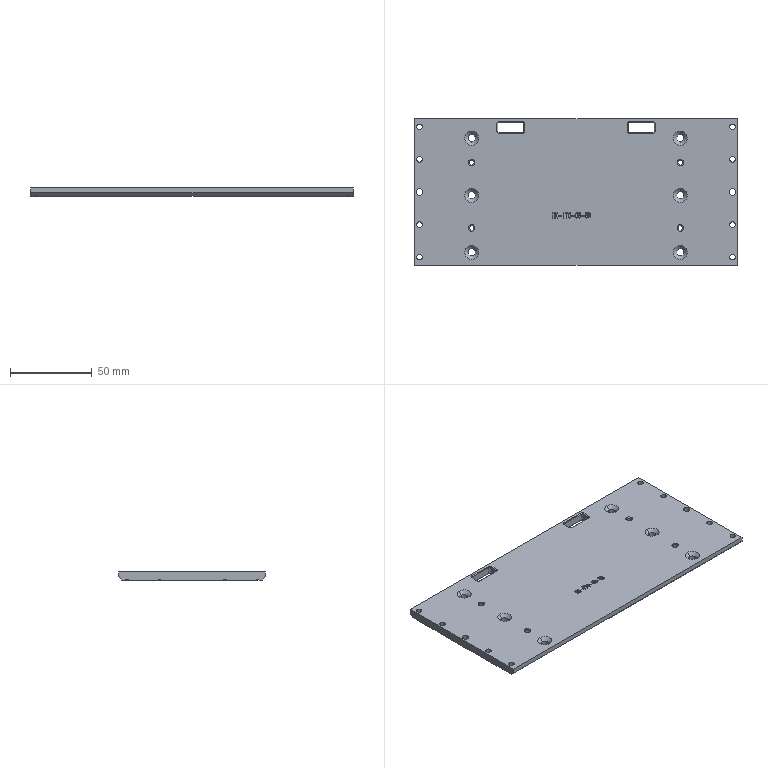Part | 1 solid | 381 faces | box 198 x 90 x 5 mm | volume 57690 mm3 | plane 174 | spline 87 | cylinder 64 | cone 56 | commonest cylinder face diameters 3.4 x16 12 x16 4.5 x12 2 x8 3 x8 4 x4